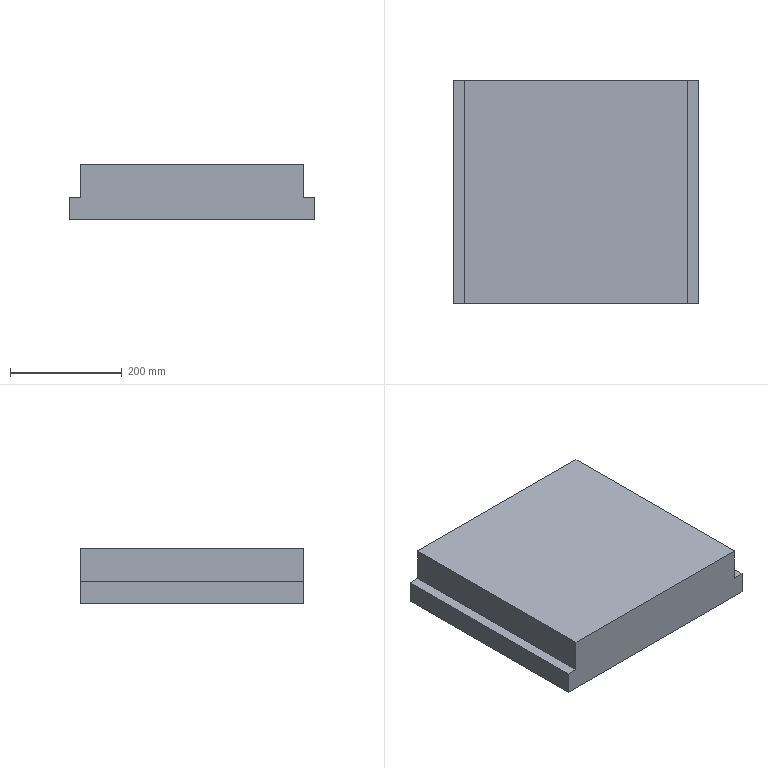Part | STEP file | Part3 | 1 solid | 10 faces | box 440 x 400 x 100 mm | volume 16640000 mm3 | plane 10
STEP:
#1=CARTESIAN_POINT('',(0.,0.,0.));
#2=DIRECTION('',(0.,0.,1.));
#3=DIRECTION('',(1.,0.,0.));
#4=AXIS2_PLACEMENT_3D('',#1,#2,#3);
#5=CARTESIAN_POINT('',(0.,0.,40.));
#6=VERTEX_POINT('',#5);
#7=CARTESIAN_POINT('',(0.,-400.,40.));
#8=VERTEX_POINT('',#7);
#9=CARTESIAN_POINT('',(0.,-100.,40.));
#10=DIRECTION('',(0.,-1.,0.));
#11=VECTOR('',#10,1.);
#12=LINE('',#9,#11);
#13=CARTESIAN_POINT('',(200.,-200.,40.));
#14=DIRECTION('',(0.,0.,1.));
#15=DIRECTION('',(1.,0.,0.));
#16=AXIS2_PLACEMENT_3D('',#13,#14,#15);
#17=PLANE('',#16);
#18=CARTESIAN_POINT('',(-200.,100.));
#19=DIRECTION('',(0.,-1.));
#20=VECTOR('',#19,1.);
#21=LINE('',#18,#20);
#22=(GEOMETRIC_REPRESENTATION_CONTEXT(2)PARAMETRIC_REPRESENTATION_CONTEXT()REPRESENTATION_CONTEXT('',''));
#23=DEFINITIONAL_REPRESENTATION('',(#21),#22);
#24=PCURVE('',#17,#23);
#25=CARTESIAN_POINT('',(0.,0.,0.));
#26=DIRECTION('',(-1.,0.,0.));
#27=DIRECTION('',(0.,-1.,0.));
#28=AXIS2_PLACEMENT_3D('',#25,#26,#27);
#29=PLANE('',#28);
#30=CARTESIAN_POINT('',(100.,40.));
#31=DIRECTION('',(1.,0.));
#32=VECTOR('',#31,1.);
#33=LINE('',#30,#32);
#34=(GEOMETRIC_REPRESENTATION_CONTEXT(2)PARAMETRIC_REPRESENTATION_CONTEXT()REPRESENTATION_CONTEXT('',''));
#35=DEFINITIONAL_REPRESENTATION('',(#33),#34);
#36=PCURVE('',#29,#35);
#37=SURFACE_CURVE('',#12,(#24,#36),.PCURVE_S1.);
#38=EDGE_CURVE('',#6,#8,#37,.T.);
#39=ORIENTED_EDGE('',*,*,#38,.F.);
#40=CARTESIAN_POINT('',(-20.,0.,40.));
#41=VERTEX_POINT('',#40);
#42=CARTESIAN_POINT('',(-20.,0.,40.));
#43=DIRECTION('',(-1.,0.,0.));
#44=VECTOR('',#43,1.);
#45=LINE('',#42,#44);
#46=CARTESIAN_POINT('',(-220.,200.));
#47=DIRECTION('',(-1.,0.));
#48=VECTOR('',#47,1.);
#49=LINE('',#46,#48);
#50=(GEOMETRIC_REPRESENTATION_CONTEXT(2)PARAMETRIC_REPRESENTATION_CONTEXT()REPRESENTATION_CONTEXT('',''));
#51=DEFINITIONAL_REPRESENTATION('',(#49),#50);
#52=PCURVE('',#17,#51);
#53=CARTESIAN_POINT('',(400.,0.,0.));
#54=DIRECTION('',(0.,1.,0.));
#55=DIRECTION('',(-1.,0.,0.));
#56=AXIS2_PLACEMENT_3D('',#53,#54,#55);
#57=PLANE('',#56);
#58=CARTESIAN_POINT('',(420.,40.));
#59=DIRECTION('',(1.,0.));
#60=VECTOR('',#59,1.);
#61=LINE('',#58,#60);
#62=(GEOMETRIC_REPRESENTATION_CONTEXT(2)PARAMETRIC_REPRESENTATION_CONTEXT()REPRESENTATION_CONTEXT('',''));
#63=DEFINITIONAL_REPRESENTATION('',(#61),#62);
#64=PCURVE('',#57,#63);
#65=SURFACE_CURVE('',#45,(#52,#64),.PCURVE_S1.);
#66=EDGE_CURVE('',#6,#41,#65,.T.);
#67=ORIENTED_EDGE('',*,*,#66,.T.);
#68=CARTESIAN_POINT('',(-20.,-400.,40.));
#69=VERTEX_POINT('',#68);
#70=CARTESIAN_POINT('',(-20.,-400.,40.));
#71=DIRECTION('',(0.,-1.,0.));
#72=VECTOR('',#71,1.);
#73=LINE('',#70,#72);
#74=CARTESIAN_POINT('',(-220.,-200.));
#75=DIRECTION('',(0.,-1.));
#76=VECTOR('',#75,1.);
#77=LINE('',#74,#76);
#78=(GEOMETRIC_REPRESENTATION_CONTEXT(2)PARAMETRIC_REPRESENTATION_CONTEXT()REPRESENTATION_CONTEXT('',''));
#79=DEFINITIONAL_REPRESENTATION('',(#77),#78);
#80=PCURVE('',#17,#79);
#81=CARTESIAN_POINT('',(-20.,0.,0.));
#82=DIRECTION('',(-1.,0.,0.));
#83=DIRECTION('',(0.,-1.,0.));
#84=AXIS2_PLACEMENT_3D('',#81,#82,#83);
#85=PLANE('',#84);
#86=CARTESIAN_POINT('',(400.,40.));
#87=DIRECTION('',(1.,0.));
#88=VECTOR('',#87,1.);
#89=LINE('',#86,#88);
#90=(GEOMETRIC_REPRESENTATION_CONTEXT(2)PARAMETRIC_REPRESENTATION_CONTEXT()REPRESENTATION_CONTEXT('',''));
#91=DEFINITIONAL_REPRESENTATION('',(#89),#90);
#92=PCURVE('',#85,#91);
#93=SURFACE_CURVE('',#73,(#80,#92),.PCURVE_S1.);
#94=EDGE_CURVE('',#41,#69,#93,.T.);
#95=ORIENTED_EDGE('',*,*,#94,.T.);
#96=CARTESIAN_POINT('',(420.,-400.,40.));
#97=DIRECTION('',(1.,0.,0.));
#98=VECTOR('',#97,1.);
#99=LINE('',#96,#98);
#100=CARTESIAN_POINT('',(220.,-200.));
#101=DIRECTION('',(1.,0.));
#102=VECTOR('',#101,1.);
#103=LINE('',#100,#102);
#104=(GEOMETRIC_REPRESENTATION_CONTEXT(2)PARAMETRIC_REPRESENTATION_CONTEXT()REPRESENTATION_CONTEXT('',''));
#105=DEFINITIONAL_REPRESENTATION('',(#103),#104);
#106=PCURVE('',#17,#105);
#107=CARTESIAN_POINT('',(0.,-400.,0.));
#108=DIRECTION('',(0.,-1.,0.));
#109=DIRECTION('',(1.,0.,0.));
#110=AXIS2_PLACEMENT_3D('',#107,#108,#109);
#111=PLANE('',#110);
#112=CARTESIAN_POINT('',(420.,40.));
#113=DIRECTION('',(1.,0.));
#114=VECTOR('',#113,1.);
#115=LINE('',#112,#114);
#116=(GEOMETRIC_REPRESENTATION_CONTEXT(2)PARAMETRIC_REPRESENTATION_CONTEXT()REPRESENTATION_CONTEXT('',''));
#117=DEFINITIONAL_REPRESENTATION('',(#115),#116);
#118=PCURVE('',#111,#117);
#119=SURFACE_CURVE('',#99,(#106,#118),.PCURVE_S1.);
#120=EDGE_CURVE('',#69,#8,#119,.T.);
#121=ORIENTED_EDGE('',*,*,#120,.T.);
#122=EDGE_LOOP('',(#39,#67,#95,#121));
#123=FACE_BOUND('',#122,.T.);
#124=ADVANCED_FACE('',(#123),#17,.T.);
#125=CARTESIAN_POINT('',(420.,0.,0.));
#126=VERTEX_POINT('',#125);
#127=CARTESIAN_POINT('',(420.,-400.,0.));
#128=VERTEX_POINT('',#127);
#129=CARTESIAN_POINT('',(420.,0.,0.));
#130=DIRECTION('',(0.,-1.,0.));
#131=VECTOR('',#130,1.);
#132=LINE('',#129,#131);
#133=CARTESIAN_POINT('',(420.,-400.,0.));
#134=DIRECTION('',(1.,0.,0.));
#135=DIRECTION('',(0.,1.,0.));
#136=AXIS2_PLACEMENT_3D('',#133,#134,#135);
#137=PLANE('',#136);
#138=CARTESIAN_POINT('',(400.,0.));
#139=DIRECTION('',(-1.,0.));
#140=VECTOR('',#139,1.);
#141=LINE('',#138,#140);
#142=(GEOMETRIC_REPRESENTATION_CONTEXT(2)PARAMETRIC_REPRESENTATION_CONTEXT()REPRESENTATION_CONTEXT('',''));
#143=DEFINITIONAL_REPRESENTATION('',(#141),#142);
#144=PCURVE('',#137,#143);
#145=CARTESIAN_POINT('',(200.,-200.,0.));
#146=DIRECTION('',(0.,0.,1.));
#147=DIRECTION('',(1.,0.,0.));
#148=AXIS2_PLACEMENT_3D('',#145,#146,#147);
#149=PLANE('',#148);
#150=CARTESIAN_POINT('',(220.,200.));
#151=DIRECTION('',(0.,-1.));
#152=VECTOR('',#151,1.);
#153=LINE('',#150,#152);
#154=(GEOMETRIC_REPRESENTATION_CONTEXT(2)PARAMETRIC_REPRESENTATION_CONTEXT()REPRESENTATION_CONTEXT('',''));
#155=DEFINITIONAL_REPRESENTATION('',(#153),#154);
#156=PCURVE('',#149,#155);
#157=SURFACE_CURVE('',#132,(#144,#156),.PCURVE_S1.);
#158=EDGE_CURVE('',#126,#128,#157,.T.);
#159=ORIENTED_EDGE('',*,*,#158,.F.);
#160=CARTESIAN_POINT('',(420.,0.,40.));
#161=VERTEX_POINT('',#160);
#162=CARTESIAN_POINT('',(420.,0.,0.));
#163=DIRECTION('',(0.,0.,1.));
#164=VECTOR('',#163,1.);
#165=LINE('',#162,#164);
#166=CARTESIAN_POINT('',(400.,0.));
#167=DIRECTION('',(0.,1.));
#168=VECTOR('',#167,1.);
#169=LINE('',#166,#168);
#170=(GEOMETRIC_REPRESENTATION_CONTEXT(2)PARAMETRIC_REPRESENTATION_CONTEXT()REPRESENTATION_CONTEXT('',''));
#171=DEFINITIONAL_REPRESENTATION('',(#169),#170);
#172=PCURVE('',#137,#171);
#173=CARTESIAN_POINT('',(-20.,0.));
#174=DIRECTION('',(0.,1.));
#175=VECTOR('',#174,1.);
#176=LINE('',#173,#175);
#177=(GEOMETRIC_REPRESENTATION_CONTEXT(2)PARAMETRIC_REPRESENTATION_CONTEXT()REPRESENTATION_CONTEXT('',''));
#178=DEFINITIONAL_REPRESENTATION('',(#176),#177);
#179=PCURVE('',#57,#178);
#180=SURFACE_CURVE('',#165,(#172,#179),.PCURVE_S1.);
#181=EDGE_CURVE('',#126,#161,#180,.T.);
#182=ORIENTED_EDGE('',*,*,#181,.T.);
#183=CARTESIAN_POINT('',(420.,-400.,40.));
#184=VERTEX_POINT('',#183);
#185=CARTESIAN_POINT('',(420.,0.,40.));
#186=DIRECTION('',(0.,1.,0.));
#187=VECTOR('',#186,1.);
#188=LINE('',#185,#187);
#189=CARTESIAN_POINT('',(400.,40.));
#190=DIRECTION('',(1.,0.));
#191=VECTOR('',#190,1.);
#192=LINE('',#189,#191);
#193=(GEOMETRIC_REPRESENTATION_CONTEXT(2)PARAMETRIC_REPRESENTATION_CONTEXT()REPRESENTATION_CONTEXT('',''));
#194=DEFINITIONAL_REPRESENTATION('',(#192),#193);
#195=PCURVE('',#137,#194);
#196=CARTESIAN_POINT('',(200.,-200.,40.));
#197=DIRECTION('',(0.,0.,1.));
#198=DIRECTION('',(1.,0.,0.));
#199=AXIS2_PLACEMENT_3D('',#196,#197,#198);
#200=PLANE('',#199);
#201=CARTESIAN_POINT('',(220.,200.));
#202=DIRECTION('',(0.,1.));
#203=VECTOR('',#202,1.);
#204=LINE('',#201,#203);
#205=(GEOMETRIC_REPRESENTATION_CONTEXT(2)PARAMETRIC_REPRESENTATION_CONTEXT()REPRESENTATION_CONTEXT('',''));
#206=DEFINITIONAL_REPRESENTATION('',(#204),#205);
#207=PCURVE('',#200,#206);
#208=SURFACE_CURVE('',#188,(#195,#207),.PCURVE_S1.);
#209=EDGE_CURVE('',#184,#161,#208,.T.);
#210=ORIENTED_EDGE('',*,*,#209,.F.);
#211=CARTESIAN_POINT('',(420.,-400.,0.));
#212=DIRECTION('',(0.,0.,1.));
#213=VECTOR('',#212,1.);
#214=LINE('',#211,#213);
#215=CARTESIAN_POINT('',(0.,0.));
#216=DIRECTION('',(0.,1.));
#217=VECTOR('',#216,1.);
#218=LINE('',#215,#217);
#219=(GEOMETRIC_REPRESENTATION_CONTEXT(2)PARAMETRIC_REPRESENTATION_CONTEXT()REPRESENTATION_CONTEXT('',''));
#220=DEFINITIONAL_REPRESENTATION('',(#218),#219);
#221=PCURVE('',#137,#220);
#222=CARTESIAN_POINT('',(420.,0.));
#223=DIRECTION('',(0.,1.));
#224=VECTOR('',#223,1.);
#225=LINE('',#222,#224);
#226=(GEOMETRIC_REPRESENTATION_CONTEXT(2)PARAMETRIC_REPRESENTATION_CONTEXT()REPRESENTATION_CONTEXT('',''));
#227=DEFINITIONAL_REPRESENTATION('',(#225),#226);
#228=PCURVE('',#111,#227);
#229=SURFACE_CURVE('',#214,(#221,#228),.PCURVE_S1.);
#230=EDGE_CURVE('',#128,#184,#229,.T.);
#231=ORIENTED_EDGE('',*,*,#230,.F.);
#232=EDGE_LOOP('',(#159,#182,#210,#231));
#233=FACE_BOUND('',#232,.T.);
#234=ADVANCED_FACE('',(#233),#137,.T.);
#235=CARTESIAN_POINT('',(-20.,-400.,0.));
#236=VERTEX_POINT('',#235);
#237=CARTESIAN_POINT('',(-20.,0.,0.));
#238=VERTEX_POINT('',#237);
#239=CARTESIAN_POINT('',(-20.,-400.,0.));
#240=DIRECTION('',(0.,1.,0.));
#241=VECTOR('',#240,1.);
#242=LINE('',#239,#241);
#243=CARTESIAN_POINT('',(400.,0.));
#244=DIRECTION('',(-1.,0.));
#245=VECTOR('',#244,1.);
#246=LINE('',#243,#245);
#247=(GEOMETRIC_REPRESENTATION_CONTEXT(2)PARAMETRIC_REPRESENTATION_CONTEXT()REPRESENTATION_CONTEXT('',''));
#248=DEFINITIONAL_REPRESENTATION('',(#246),#247);
#249=PCURVE('',#85,#248);
#250=CARTESIAN_POINT('',(-220.,-200.));
#251=DIRECTION('',(0.,1.));
#252=VECTOR('',#251,1.);
#253=LINE('',#250,#252);
#254=(GEOMETRIC_REPRESENTATION_CONTEXT(2)PARAMETRIC_REPRESENTATION_CONTEXT()REPRESENTATION_CONTEXT('',''));
#255=DEFINITIONAL_REPRESENTATION('',(#253),#254);
#256=PCURVE('',#149,#255);
#257=SURFACE_CURVE('',#242,(#249,#256),.PCURVE_S1.);
#258=EDGE_CURVE('',#236,#238,#257,.T.);
#259=ORIENTED_EDGE('',*,*,#258,.F.);
#260=CARTESIAN_POINT('',(-20.,-400.,0.));
#261=DIRECTION('',(0.,0.,1.));
#262=VECTOR('',#261,1.);
#263=LINE('',#260,#262);
#264=CARTESIAN_POINT('',(400.,0.));
#265=DIRECTION('',(0.,1.));
#266=VECTOR('',#265,1.);
#267=LINE('',#264,#266);
#268=(GEOMETRIC_REPRESENTATION_CONTEXT(2)PARAMETRIC_REPRESENTATION_CONTEXT()REPRESENTATION_CONTEXT('',''));
#269=DEFINITIONAL_REPRESENTATION('',(#267),#268);
#270=PCURVE('',#85,#269);
#271=CARTESIAN_POINT('',(-20.,0.));
#272=DIRECTION('',(0.,1.));
#273=VECTOR('',#272,1.);
#274=LINE('',#271,#273);
#275=(GEOMETRIC_REPRESENTATION_CONTEXT(2)PARAMETRIC_REPRESENTATION_CONTEXT()REPRESENTATION_CONTEXT('',''));
#276=DEFINITIONAL_REPRESENTATION('',(#274),#275);
#277=PCURVE('',#111,#276);
#278=SURFACE_CURVE('',#263,(#270,#277),.PCURVE_S1.);
#279=EDGE_CURVE('',#236,#69,#278,.T.);
#280=ORIENTED_EDGE('',*,*,#279,.T.);
#281=ORIENTED_EDGE('',*,*,#94,.F.);
#282=CARTESIAN_POINT('',(-20.,0.,0.));
#283=DIRECTION('',(0.,0.,1.));
#284=VECTOR('',#283,1.);
#285=LINE('',#282,#284);
#286=CARTESIAN_POINT('',(0.,0.));
#287=DIRECTION('',(0.,1.));
#288=VECTOR('',#287,1.);
#289=LINE('',#286,#288);
#290=(GEOMETRIC_REPRESENTATION_CONTEXT(2)PARAMETRIC_REPRESENTATION_CONTEXT()REPRESENTATION_CONTEXT('',''));
#291=DEFINITIONAL_REPRESENTATION('',(#289),#290);
#292=PCURVE('',#85,#291);
#293=CARTESIAN_POINT('',(420.,0.));
#294=DIRECTION('',(0.,1.));
#295=VECTOR('',#294,1.);
#296=LINE('',#293,#295);
#297=(GEOMETRIC_REPRESENTATION_CONTEXT(2)PARAMETRIC_REPRESENTATION_CONTEXT()REPRESENTATION_CONTEXT('',''));
#298=DEFINITIONAL_REPRESENTATION('',(#296),#297);
#299=PCURVE('',#57,#298);
#300=SURFACE_CURVE('',#285,(#292,#299),.PCURVE_S1.);
#301=EDGE_CURVE('',#238,#41,#300,.T.);
#302=ORIENTED_EDGE('',*,*,#301,.F.);
#303=EDGE_LOOP('',(#259,#280,#281,#302));
#304=FACE_BOUND('',#303,.T.);
#305=ADVANCED_FACE('',(#304),#85,.T.);
#306=CARTESIAN_POINT('',(400.,-400.,40.));
#307=VERTEX_POINT('',#306);
#308=CARTESIAN_POINT('',(400.,0.,40.));
#309=VERTEX_POINT('',#308);
#310=CARTESIAN_POINT('',(400.,-300.,40.));
#311=DIRECTION('',(0.,1.,0.));
#312=VECTOR('',#311,1.);
#313=LINE('',#310,#312);
#314=CARTESIAN_POINT('',(200.,-100.));
#315=DIRECTION('',(0.,1.));
#316=VECTOR('',#315,1.);
#317=LINE('',#314,#316);
#318=(GEOMETRIC_REPRESENTATION_CONTEXT(2)PARAMETRIC_REPRESENTATION_CONTEXT()REPRESENTATION_CONTEXT('',''));
#319=DEFINITIONAL_REPRESENTATION('',(#317),#318);
#320=PCURVE('',#200,#319);
#321=CARTESIAN_POINT('',(400.,-400.,0.));
#322=DIRECTION('',(1.,0.,0.));
#323=DIRECTION('',(0.,1.,0.));
#324=AXIS2_PLACEMENT_3D('',#321,#322,#323);
#325=PLANE('',#324);
#326=CARTESIAN_POINT('',(100.,40.));
#327=DIRECTION('',(1.,0.));
#328=VECTOR('',#327,1.);
#329=LINE('',#326,#328);
#330=(GEOMETRIC_REPRESENTATION_CONTEXT(2)PARAMETRIC_REPRESENTATION_CONTEXT()REPRESENTATION_CONTEXT('',''));
#331=DEFINITIONAL_REPRESENTATION('',(#329),#330);
#332=PCURVE('',#325,#331);
#333=SURFACE_CURVE('',#313,(#320,#332),.PCURVE_S1.);
#334=EDGE_CURVE('',#307,#309,#333,.T.);
#335=ORIENTED_EDGE('',*,*,#334,.F.);
#336=CARTESIAN_POINT('',(420.,-400.,40.));
#337=DIRECTION('',(1.,0.,0.));
#338=VECTOR('',#337,1.);
#339=LINE('',#336,#338);
#340=CARTESIAN_POINT('',(220.,-200.));
#341=DIRECTION('',(1.,0.));
#342=VECTOR('',#341,1.);
#343=LINE('',#340,#342);
#344=(GEOMETRIC_REPRESENTATION_CONTEXT(2)PARAMETRIC_REPRESENTATION_CONTEXT()REPRESENTATION_CONTEXT('',''));
#345=DEFINITIONAL_REPRESENTATION('',(#343),#344);
#346=PCURVE('',#200,#345);
#347=CARTESIAN_POINT('',(420.,40.));
#348=DIRECTION('',(1.,0.));
#349=VECTOR('',#348,1.);
#350=LINE('',#347,#349);
#351=(GEOMETRIC_REPRESENTATION_CONTEXT(2)PARAMETRIC_REPRESENTATION_CONTEXT()REPRESENTATION_CONTEXT('',''));
#352=DEFINITIONAL_REPRESENTATION('',(#350),#351);
#353=PCURVE('',#111,#352);
#354=SURFACE_CURVE('',#339,(#346,#353),.PCURVE_S1.);
#355=EDGE_CURVE('',#307,#184,#354,.T.);
#356=ORIENTED_EDGE('',*,*,#355,.T.);
#357=ORIENTED_EDGE('',*,*,#209,.T.);
#358=CARTESIAN_POINT('',(-20.,0.,40.));
#359=DIRECTION('',(-1.,0.,0.));
#360=VECTOR('',#359,1.);
#361=LINE('',#358,#360);
#362=CARTESIAN_POINT('',(-220.,200.));
#363=DIRECTION('',(-1.,0.));
#364=VECTOR('',#363,1.);
#365=LINE('',#362,#364);
#366=(GEOMETRIC_REPRESENTATION_CONTEXT(2)PARAMETRIC_REPRESENTATION_CONTEXT()REPRESENTATION_CONTEXT('',''));
#367=DEFINITIONAL_REPRESENTATION('',(#365),#366);
#368=PCURVE('',#200,#367);
#369=CARTESIAN_POINT('',(420.,40.));
#370=DIRECTION('',(1.,0.));
#371=VECTOR('',#370,1.);
#372=LINE('',#369,#371);
#373=(GEOMETRIC_REPRESENTATION_CONTEXT(2)PARAMETRIC_REPRESENTATION_CONTEXT()REPRESENTATION_CONTEXT('',''));
#374=DEFINITIONAL_REPRESENTATION('',(#372),#373);
#375=PCURVE('',#57,#374);
#376=SURFACE_CURVE('',#361,(#368,#375),.PCURVE_S1.);
#377=EDGE_CURVE('',#161,#309,#376,.T.);
#378=ORIENTED_EDGE('',*,*,#377,.T.);
#379=EDGE_LOOP('',(#335,#356,#357,#378));
#380=FACE_BOUND('',#379,.T.);
#381=ADVANCED_FACE('',(#380),#200,.T.);
#382=ORIENTED_EDGE('',*,*,#334,.T.);
#383=CARTESIAN_POINT('',(400.,0.,100.));
#384=VERTEX_POINT('',#383);
#385=CARTESIAN_POINT('',(400.,0.,0.));
#386=DIRECTION('',(0.,0.,1.));
#387=VECTOR('',#386,1.);
#388=LINE('',#385,#387);
#389=CARTESIAN_POINT('',(400.,0.));
#390=DIRECTION('',(0.,1.));
#391=VECTOR('',#390,1.);
#392=LINE('',#389,#391);
#393=(GEOMETRIC_REPRESENTATION_CONTEXT(2)PARAMETRIC_REPRESENTATION_CONTEXT()REPRESENTATION_CONTEXT('',''));
#394=DEFINITIONAL_REPRESENTATION('',(#392),#393);
#395=PCURVE('',#325,#394);
#396=CARTESIAN_POINT('',(0.,0.));
#397=DIRECTION('',(0.,1.));
#398=VECTOR('',#397,1.);
#399=LINE('',#396,#398);
#400=(GEOMETRIC_REPRESENTATION_CONTEXT(2)PARAMETRIC_REPRESENTATION_CONTEXT()REPRESENTATION_CONTEXT('',''));
#401=DEFINITIONAL_REPRESENTATION('',(#399),#400);
#402=PCURVE('',#57,#401);
#403=SURFACE_CURVE('',#388,(#395,#402),.PCURVE_S1.);
#404=EDGE_CURVE('',#309,#384,#403,.T.);
#405=ORIENTED_EDGE('',*,*,#404,.T.);
#406=CARTESIAN_POINT('',(400.,-400.,100.));
#407=VERTEX_POINT('',#406);
#408=CARTESIAN_POINT('',(400.,0.,100.));
#409=DIRECTION('',(0.,1.,0.));
#410=VECTOR('',#409,1.);
#411=LINE('',#408,#410);
#412=CARTESIAN_POINT('',(400.,100.));
#413=DIRECTION('',(1.,0.));
#414=VECTOR('',#413,1.);
#415=LINE('',#412,#414);
#416=(GEOMETRIC_REPRESENTATION_CONTEXT(2)PARAMETRIC_REPRESENTATION_CONTEXT()REPRESENTATION_CONTEXT('',''));
#417=DEFINITIONAL_REPRESENTATION('',(#415),#416);
#418=PCURVE('',#325,#417);
#419=CARTESIAN_POINT('',(200.,-200.,100.));
#420=DIRECTION('',(0.,0.,1.));
#421=DIRECTION('',(1.,0.,0.));
#422=AXIS2_PLACEMENT_3D('',#419,#420,#421);
#423=PLANE('',#422);
#424=CARTESIAN_POINT('',(200.,200.));
#425=DIRECTION('',(0.,1.));
#426=VECTOR('',#425,1.);
#427=LINE('',#424,#426);
#428=(GEOMETRIC_REPRESENTATION_CONTEXT(2)PARAMETRIC_REPRESENTATION_CONTEXT()REPRESENTATION_CONTEXT('',''));
#429=DEFINITIONAL_REPRESENTATION('',(#427),#428);
#430=PCURVE('',#423,#429);
#431=SURFACE_CURVE('',#411,(#418,#430),.PCURVE_S1.);
#432=EDGE_CURVE('',#407,#384,#431,.T.);
#433=ORIENTED_EDGE('',*,*,#432,.F.);
#434=CARTESIAN_POINT('',(400.,-400.,0.));
#435=DIRECTION('',(0.,0.,1.));
#436=VECTOR('',#435,1.);
#437=LINE('',#434,#436);
#438=CARTESIAN_POINT('',(0.,0.));
#439=DIRECTION('',(0.,1.));
#440=VECTOR('',#439,1.);
#441=LINE('',#438,#440);
#442=(GEOMETRIC_REPRESENTATION_CONTEXT(2)PARAMETRIC_REPRESENTATION_CONTEXT()REPRESENTATION_CONTEXT('',''));
#443=DEFINITIONAL_REPRESENTATION('',(#441),#442);
#444=PCURVE('',#325,#443);
#445=CARTESIAN_POINT('',(400.,0.));
#446=DIRECTION('',(0.,1.));
#447=VECTOR('',#446,1.);
#448=LINE('',#445,#447);
#449=(GEOMETRIC_REPRESENTATION_CONTEXT(2)PARAMETRIC_REPRESENTATION_CONTEXT()REPRESENTATION_CONTEXT('',''));
#450=DEFINITIONAL_REPRESENTATION('',(#448),#449);
#451=PCURVE('',#111,#450);
#452=SURFACE_CURVE('',#437,(#444,#451),.PCURVE_S1.);
#453=EDGE_CURVE('',#307,#407,#452,.T.);
#454=ORIENTED_EDGE('',*,*,#453,.F.);
#455=EDGE_LOOP('',(#382,#405,#433,#454));
#456=FACE_BOUND('',#455,.T.);
#457=ADVANCED_FACE('',(#456),#325,.T.);
#458=CARTESIAN_POINT('',(0.,0.,100.));
#459=VERTEX_POINT('',#458);
#460=CARTESIAN_POINT('',(0.,0.,0.));
#461=DIRECTION('',(0.,0.,1.));
#462=VECTOR('',#461,1.);
#463=LINE('',#460,#462);
#464=CARTESIAN_POINT('',(400.,0.));
#465=DIRECTION('',(0.,1.));
#466=VECTOR('',#465,1.);
#467=LINE('',#464,#466);
#468=(GEOMETRIC_REPRESENTATION_CONTEXT(2)PARAMETRIC_REPRESENTATION_CONTEXT()REPRESENTATION_CONTEXT('',''));
#469=DEFINITIONAL_REPRESENTATION('',(#467),#468);
#470=PCURVE('',#57,#469);
#471=CARTESIAN_POINT('',(0.,0.));
#472=DIRECTION('',(0.,1.));
#473=VECTOR('',#472,1.);
#474=LINE('',#471,#473);
#475=(GEOMETRIC_REPRESENTATION_CONTEXT(2)PARAMETRIC_REPRESENTATION_CONTEXT()REPRESENTATION_CONTEXT('',''));
#476=DEFINITIONAL_REPRESENTATION('',(#474),#475);
#477=PCURVE('',#29,#476);
#478=SURFACE_CURVE('',#463,(#470,#477),.PCURVE_S1.);
#479=EDGE_CURVE('',#6,#459,#478,.T.);
#480=ORIENTED_EDGE('',*,*,#479,.T.);
#481=CARTESIAN_POINT('',(0.,0.,100.));
#482=DIRECTION('',(-1.,0.,0.));
#483=VECTOR('',#482,1.);
#484=LINE('',#481,#483);
#485=CARTESIAN_POINT('',(400.,100.));
#486=DIRECTION('',(1.,0.));
#487=VECTOR('',#486,1.);
#488=LINE('',#485,#487);
#489=(GEOMETRIC_REPRESENTATION_CONTEXT(2)PARAMETRIC_REPRESENTATION_CONTEXT()REPRESENTATION_CONTEXT('',''));
#490=DEFINITIONAL_REPRESENTATION('',(#488),#489);
#491=PCURVE('',#57,#490);
#492=CARTESIAN_POINT('',(-200.,200.));
#493=DIRECTION('',(-1.,0.));
#494=VECTOR('',#493,1.);
#495=LINE('',#492,#494);
#496=(GEOMETRIC_REPRESENTATION_CONTEXT(2)PARAMETRIC_REPRESENTATION_CONTEXT()REPRESENTATION_CONTEXT('',''));
#497=DEFINITIONAL_REPRESENTATION('',(#495),#496);
#498=PCURVE('',#423,#497);
#499=SURFACE_CURVE('',#484,(#491,#498),.PCURVE_S1.);
#500=EDGE_CURVE('',#384,#459,#499,.T.);
#501=ORIENTED_EDGE('',*,*,#500,.F.);
#502=ORIENTED_EDGE('',*,*,#404,.F.);
#503=ORIENTED_EDGE('',*,*,#377,.F.);
#504=ORIENTED_EDGE('',*,*,#181,.F.);
#505=CARTESIAN_POINT('',(0.,0.,0.));
#506=DIRECTION('',(1.,0.,0.));
#507=VECTOR('',#506,1.);
#508=LINE('',#505,#507);
#509=CARTESIAN_POINT('',(400.,0.));
#510=DIRECTION('',(-1.,0.));
#511=VECTOR('',#510,1.);
#512=LINE('',#509,#511);
#513=(GEOMETRIC_REPRESENTATION_CONTEXT(2)PARAMETRIC_REPRESENTATION_CONTEXT()REPRESENTATION_CONTEXT('',''));
#514=DEFINITIONAL_REPRESENTATION('',(#512),#513);
#515=PCURVE('',#57,#514);
#516=CARTESIAN_POINT('',(-200.,200.));
#517=DIRECTION('',(1.,0.));
#518=VECTOR('',#517,1.);
#519=LINE('',#516,#518);
#520=(GEOMETRIC_REPRESENTATION_CONTEXT(2)PARAMETRIC_REPRESENTATION_CONTEXT()REPRESENTATION_CONTEXT('',''));
#521=DEFINITIONAL_REPRESENTATION('',(#519),#520);
#522=PCURVE('',#149,#521);
#523=SURFACE_CURVE('',#508,(#515,#522),.PCURVE_S1.);
#524=EDGE_CURVE('',#238,#126,#523,.T.);
#525=ORIENTED_EDGE('',*,*,#524,.F.);
#526=ORIENTED_EDGE('',*,*,#301,.T.);
#527=ORIENTED_EDGE('',*,*,#66,.F.);
#528=EDGE_LOOP('',(#480,#501,#502,#503,#504,#525,#526,#527));
#529=FACE_BOUND('',#528,.T.);
#530=ADVANCED_FACE('',(#529),#57,.T.);
#531=ORIENTED_EDGE('',*,*,#453,.T.);
#532=CARTESIAN_POINT('',(0.,-400.,100.));
#533=VERTEX_POINT('',#532);
#534=CARTESIAN_POINT('',(400.,-400.,100.));
#535=DIRECTION('',(1.,0.,0.));
#536=VECTOR('',#535,1.);
#537=LINE('',#534,#536);
#538=CARTESIAN_POINT('',(400.,100.));
#539=DIRECTION('',(1.,0.));
#540=VECTOR('',#539,1.);
#541=LINE('',#538,#540);
#542=(GEOMETRIC_REPRESENTATION_CONTEXT(2)PARAMETRIC_REPRESENTATION_CONTEXT()REPRESENTATION_CONTEXT('',''));
#543=DEFINITIONAL_REPRESENTATION('',(#541),#542);
#544=PCURVE('',#111,#543);
#545=CARTESIAN_POINT('',(200.,-200.));
#546=DIRECTION('',(1.,0.));
#547=VECTOR('',#546,1.);
#548=LINE('',#545,#547);
#549=(GEOMETRIC_REPRESENTATION_CONTEXT(2)PARAMETRIC_REPRESENTATION_CONTEXT()REPRESENTATION_CONTEXT('',''));
#550=DEFINITIONAL_REPRESENTATION('',(#548),#549);
#551=PCURVE('',#423,#550);
#552=SURFACE_CURVE('',#537,(#544,#551),.PCURVE_S1.);
#553=EDGE_CURVE('',#533,#407,#552,.T.);
#554=ORIENTED_EDGE('',*,*,#553,.F.);
#555=CARTESIAN_POINT('',(0.,-400.,0.));
#556=DIRECTION('',(0.,0.,1.));
#557=VECTOR('',#556,1.);
#558=LINE('',#555,#557);
#559=CARTESIAN_POINT('',(0.,0.));
#560=DIRECTION('',(0.,1.));
#561=VECTOR('',#560,1.);
#562=LINE('',#559,#561);
#563=(GEOMETRIC_REPRESENTATION_CONTEXT(2)PARAMETRIC_REPRESENTATION_CONTEXT()REPRESENTATION_CONTEXT('',''));
#564=DEFINITIONAL_REPRESENTATION('',(#562),#563);
#565=PCURVE('',#111,#564);
#566=CARTESIAN_POINT('',(400.,0.));
#567=DIRECTION('',(0.,1.));
#568=VECTOR('',#567,1.);
#569=LINE('',#566,#568);
#570=(GEOMETRIC_REPRESENTATION_CONTEXT(2)PARAMETRIC_REPRESENTATION_CONTEXT()REPRESENTATION_CONTEXT('',''));
#571=DEFINITIONAL_REPRESENTATION('',(#569),#570);
#572=PCURVE('',#29,#571);
#573=SURFACE_CURVE('',#558,(#565,#572),.PCURVE_S1.);
#574=EDGE_CURVE('',#8,#533,#573,.T.);
#575=ORIENTED_EDGE('',*,*,#574,.F.);
#576=ORIENTED_EDGE('',*,*,#120,.F.);
#577=ORIENTED_EDGE('',*,*,#279,.F.);
#578=CARTESIAN_POINT('',(400.,-400.,0.));
#579=DIRECTION('',(-1.,0.,0.));
#580=VECTOR('',#579,1.);
#581=LINE('',#578,#580);
#582=CARTESIAN_POINT('',(400.,0.));
#583=DIRECTION('',(-1.,0.));
#584=VECTOR('',#583,1.);
#585=LINE('',#582,#584);
#586=(GEOMETRIC_REPRESENTATION_CONTEXT(2)PARAMETRIC_REPRESENTATION_CONTEXT()REPRESENTATION_CONTEXT('',''));
#587=DEFINITIONAL_REPRESENTATION('',(#585),#586);
#588=PCURVE('',#111,#587);
#589=CARTESIAN_POINT('',(200.,-200.));
#590=DIRECTION('',(-1.,0.));
#591=VECTOR('',#590,1.);
#592=LINE('',#589,#591);
#593=(GEOMETRIC_REPRESENTATION_CONTEXT(2)PARAMETRIC_REPRESENTATION_CONTEXT()REPRESENTATION_CONTEXT('',''));
#594=DEFINITIONAL_REPRESENTATION('',(#592),#593);
#595=PCURVE('',#149,#594);
#596=SURFACE_CURVE('',#581,(#588,#595),.PCURVE_S1.);
#597=EDGE_CURVE('',#128,#236,#596,.T.);
#598=ORIENTED_EDGE('',*,*,#597,.F.);
#599=ORIENTED_EDGE('',*,*,#230,.T.);
#600=ORIENTED_EDGE('',*,*,#355,.F.);
#601=EDGE_LOOP('',(#531,#554,#575,#576,#577,#598,#599,#600));
#602=FACE_BOUND('',#601,.T.);
#603=ADVANCED_FACE('',(#602),#111,.T.);
#604=ORIENTED_EDGE('',*,*,#38,.T.);
#605=ORIENTED_EDGE('',*,*,#574,.T.);
#606=CARTESIAN_POINT('',(0.,-400.,100.));
#607=DIRECTION('',(0.,-1.,0.));
#608=VECTOR('',#607,1.);
#609=LINE('',#606,#608);
#610=CARTESIAN_POINT('',(400.,100.));
#611=DIRECTION('',(1.,0.));
#612=VECTOR('',#611,1.);
#613=LINE('',#610,#612);
#614=(GEOMETRIC_REPRESENTATION_CONTEXT(2)PARAMETRIC_REPRESENTATION_CONTEXT()REPRESENTATION_CONTEXT('',''));
#615=DEFINITIONAL_REPRESENTATION('',(#613),#614);
#616=PCURVE('',#29,#615);
#617=CARTESIAN_POINT('',(-200.,-200.));
#618=DIRECTION('',(0.,-1.));
#619=VECTOR('',#618,1.);
#620=LINE('',#617,#619);
#621=(GEOMETRIC_REPRESENTATION_CONTEXT(2)PARAMETRIC_REPRESENTATION_CONTEXT()REPRESENTATION_CONTEXT('',''));
#622=DEFINITIONAL_REPRESENTATION('',(#620),#621);
#623=PCURVE('',#423,#622);
#624=SURFACE_CURVE('',#609,(#616,#623),.PCURVE_S1.);
#625=EDGE_CURVE('',#459,#533,#624,.T.);
#626=ORIENTED_EDGE('',*,*,#625,.F.);
#627=ORIENTED_EDGE('',*,*,#479,.F.);
#628=EDGE_LOOP('',(#604,#605,#626,#627));
#629=FACE_BOUND('',#628,.T.);
#630=ADVANCED_FACE('',(#629),#29,.T.);
#631=ORIENTED_EDGE('',*,*,#524,.T.);
#632=ORIENTED_EDGE('',*,*,#158,.T.);
#633=ORIENTED_EDGE('',*,*,#597,.T.);
#634=ORIENTED_EDGE('',*,*,#258,.T.);
#635=EDGE_LOOP('',(#631,#632,#633,#634));
#636=FACE_BOUND('',#635,.T.);
#637=ADVANCED_FACE('',(#636),#149,.F.);
#638=ORIENTED_EDGE('',*,*,#500,.T.);
#639=ORIENTED_EDGE('',*,*,#625,.T.);
#640=ORIENTED_EDGE('',*,*,#553,.T.);
#641=ORIENTED_EDGE('',*,*,#432,.T.);
#642=EDGE_LOOP('',(#638,#639,#640,#641));
#643=FACE_BOUND('',#642,.T.);
#644=ADVANCED_FACE('',(#643),#423,.T.);
#645=CLOSED_SHELL('',(#124,#234,#305,#381,#457,#530,#603,#630,#637,#644));
#646=MANIFOLD_SOLID_BREP('',#645);
#647=(LENGTH_UNIT()NAMED_UNIT(*)SI_UNIT(.MILLI.,.METRE.));
#648=UNCERTAINTY_MEASURE_WITH_UNIT(LENGTH_MEASURE(0.0000001),#647,'','');
#649=(NAMED_UNIT(*)PLANE_ANGLE_UNIT()SI_UNIT($,.RADIAN.));
#650=(NAMED_UNIT(*)SI_UNIT($,.STERADIAN.)SOLID_ANGLE_UNIT());
#651=(GEOMETRIC_REPRESENTATION_CONTEXT(3)GLOBAL_UNCERTAINTY_ASSIGNED_CONTEXT((#648))GLOBAL_UNIT_ASSIGNED_CONTEXT((#647,#649,#650))REPRESENTATION_CONTEXT('',''));
#652=ADVANCED_BREP_SHAPE_REPRESENTATION('',(#4,#646),#651);